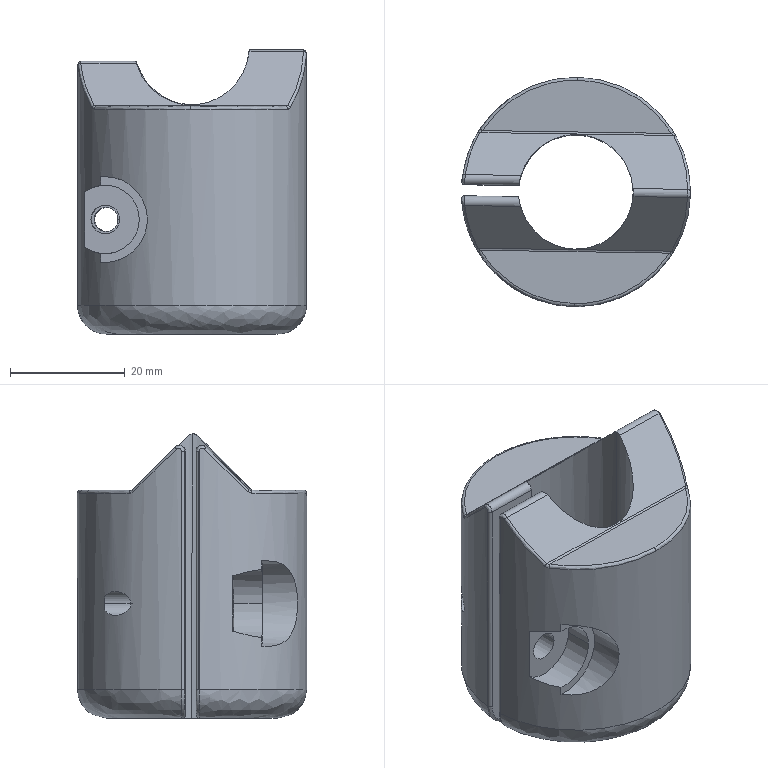Part | SolidWorks | features BaseBody 1 | 1 solid | 50 faces | box 39.963 x 40 x 49.586 mm | volume 36997 mm3 | cylinder 21 | spline 19 | plane 10 | commonest cylinder face diameters 1 x7 2 x3 4.2 x2 5 x2 12 x2 20 x2